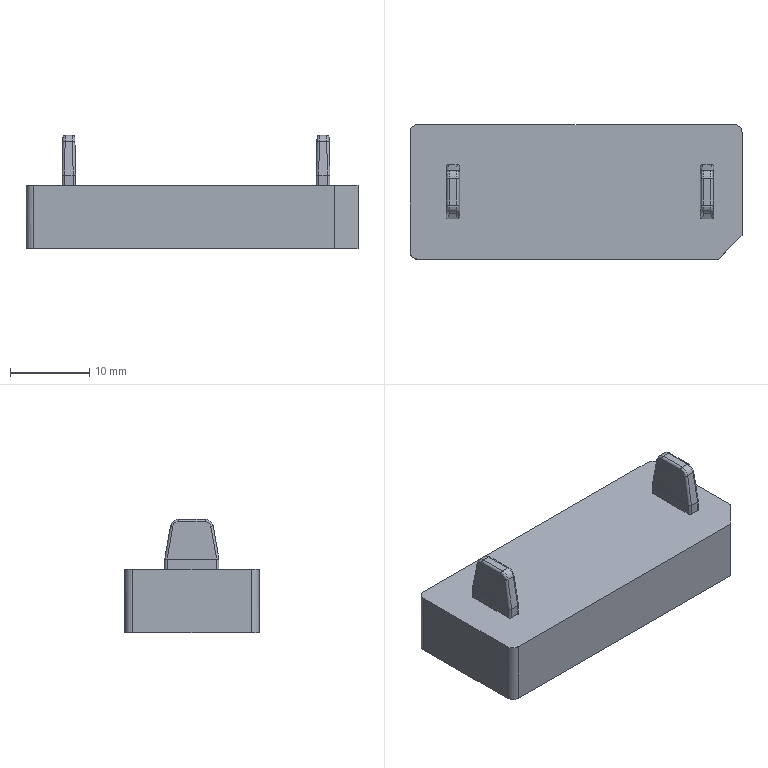NC program | PowerMill | posted by the shop | part box 42 x 17 x 14.346 mm
Lines 3988 to 5032 of 50900:
( TOOL ID   R1_2 )
( TOOL DIA. 2. TIP RAD 1. LENGTH 57. )
( Z = -2.15 )
T4 M6
T5
G91 G28 Z0
G0 G90 G54
M08
S18000 M3
X0 Y0 M8
G43 Z10.796 H4
X17.949 Y-3.022
Z-.902
G1 Z-2.102 F1200
X17.941 Y-3.03 Z-2.084 F2000
X17.924 Y-3.048 Z-2.051
X17.9 Y-3.071 Z-2.022
X17.871 Y-3.1 Z-1.995
X17.836 Y-3.136 Z-1.972
X17.82 Y-3.151 Z-1.974
X17.787 Y-3.185 Z-1.984
X17.755 Y-3.217 Z-2.002
X17.725 Y-3.246 Z-2.027
X17.699 Y-3.272 Z-2.059
X17.567 Y-3.353 Z-2.043
X17.603 Y-3.318 Z-1.96
X17.63 Y-3.29 Z-1.904
X17.656 Y-3.264 Z-1.861
X17.683 Y-3.238 Z-1.827
X17.71 Y-3.21 Z-1.801
X17.74 Y-3.181 Z-1.782
X17.771 Y-3.15 Z-1.77
X17.78 Y-3.14 Z-1.767
X17.869 Y-3.051 Z-1.781
X17.897 Y-3.023 Z-1.802
X17.923 Y-2.998 Z-1.83
X17.946 Y-2.974 Z-1.864
X17.968 Y-2.953 Z-1.907
X17.987 Y-2.933 Z-1.959
X18.006 Y-2.914 Z-2.024
X18.027 Y-2.894 Z-2.112
X18.029 Y-2.891 Z-2.122
X18.07 Y-2.799 Z-2.132
X18.063 Y-2.806 Z-2.079
X18.049 Y-2.821 Z-1.986
X18.033 Y-2.837 Z-1.913
X18.015 Y-2.855 Z-1.851
X17.994 Y-2.876 Z-1.797
X17.972 Y-2.897 Z-1.754
X17.947 Y-2.923 Z-1.716
X17.918 Y-2.952 Z-1.684
X17.886 Y-2.984 Z-1.659
X17.852 Y-3.018 Z-1.641
X17.817 Y-3.052 Z-1.631
X17.782 Y-3.087 Z-1.629
X17.748 Y-3.122 Z-1.635
X17.715 Y-3.155 Z-1.648
X17.678 Y-3.192 Z-1.669
X17.643 Y-3.226 Z-1.695
X17.612 Y-3.258 Z-1.727
X17.583 Y-3.287 Z-1.766
X17.556 Y-3.314 Z-1.811
X17.531 Y-3.339 Z-1.866
X17.506 Y-3.364 Z-1.933
X17.477 Y-3.393 Z-2.025
X17.396 Y-3.422 Z-2.013
X17.423 Y-3.395 Z-1.917
X17.449 Y-3.37 Z-1.839
X17.475 Y-3.344 Z-1.777
X17.501 Y-3.318 Z-1.726
X17.519 Y-3.3 Z-1.697
X17.543 Y-3.276 Z-1.663
X17.579 Y-3.24 Z-1.619
X17.608 Y-3.211 Z-1.591
X17.631 Y-3.188 Z-1.573
X17.656 Y-3.163 Z-1.558
X17.684 Y-3.135 Z-1.544
X17.715 Y-3.104 Z-1.53
X17.744 Y-3.075 Z-1.523
X17.772 Y-3.046 Z-1.521
X17.801 Y-3.017 Z-1.523
X17.827 Y-2.991 Z-1.529
X17.858 Y-2.96 Z-1.542
X17.894 Y-2.924 Z-1.56
X17.928 Y-2.89 Z-1.59
X17.959 Y-2.859 Z-1.625
X17.987 Y-2.831 Z-1.668
X18.012 Y-2.806 Z-1.716
X18.035 Y-2.784 Z-1.773
X18.054 Y-2.765 Z-1.838
X18.071 Y-2.748 Z-1.913
X18.085 Y-2.734 Z-2.001
X18.097 Y-2.722 Z-2.108
X18.099 Y-2.72 Z-2.134
X18.117 Y-2.651 Z-2.137
X18.113 Y-2.654 Z-2.082
X18.103 Y-2.664 Z-1.97
X18.091 Y-2.677 Z-1.878
X18.076 Y-2.692 Z-1.799
X18.058 Y-2.71 Z-1.732
X18.035 Y-2.733 Z-1.669
X18.009 Y-2.758 Z-1.614
X17.981 Y-2.787 Z-1.565
X17.949 Y-2.818 Z-1.524
X17.916 Y-2.852 Z-1.491
X17.881 Y-2.887 Z-1.465
X17.844 Y-2.924 Z-1.446
X17.805 Y-2.963 Z-1.434
X17.765 Y-3.003 Z-1.429
X17.723 Y-3.045 Z-1.432
X17.68 Y-3.088 Z-1.443
X17.638 Y-3.13 Z-1.461
X17.596 Y-3.172 Z-1.488
X17.554 Y-3.214 Z-1.523
X17.514 Y-3.254 Z-1.566
X17.477 Y-3.291 Z-1.615
X17.444 Y-3.324 Z-1.667
X17.414 Y-3.354 Z-1.724
X17.387 Y-3.381 Z-1.789
X17.363 Y-3.405 Z-1.862
X17.342 Y-3.426 Z-1.94
X17.324 Y-3.444 Z-2.019
X17.256 Y-3.461 Z-2.025
X17.278 Y-3.439 Z-1.925
X17.302 Y-3.415 Z-1.835
X17.329 Y-3.388 Z-1.753
X17.358 Y-3.359 Z-1.681
X17.39 Y-3.327 Z-1.616
X17.425 Y-3.292 Z-1.558
X17.463 Y-3.254 Z-1.507
X17.504 Y-3.213 Z-1.464
X17.548 Y-3.169 Z-1.426
X17.594 Y-3.123 Z-1.395
X17.638 Y-3.078 Z-1.373
X17.683 Y-3.034 Z-1.358
X17.727 Y-2.99 Z-1.35
X17.77 Y-2.947 Z-1.351
X17.812 Y-2.904 Z-1.359
X17.853 Y-2.864 Z-1.374
X17.893 Y-2.824 Z-1.397
X17.93 Y-2.787 Z-1.428
X17.964 Y-2.753 Z-1.466
X17.996 Y-2.721 Z-1.511
X18.025 Y-2.692 Z-1.562
X18.05 Y-2.667 Z-1.619
X18.071 Y-2.646 Z-1.682
X18.088 Y-2.629 Z-1.749
X18.102 Y-2.615 Z-1.825
X18.115 Y-2.602 Z-1.919
X18.125 Y-2.592 Z-2.028
X18.13 Y-2.587 Z-2.108
X18.137 Y-2.529 Z-2.075
Z-2.065
X18.13 Y-2.536 Z-1.951
X18.12 Y-2.546 Z-1.846
X18.107 Y-2.559 Z-1.755
X18.091 Y-2.575 Z-1.675
X18.071 Y-2.595 Z-1.604
X18.048 Y-2.618 Z-1.541
X18.022 Y-2.644 Z-1.486
X17.993 Y-2.673 Z-1.437
X17.961 Y-2.705 Z-1.395
X17.926 Y-2.74 Z-1.36
X17.888 Y-2.778 Z-1.33
X17.847 Y-2.819 Z-1.306
X17.805 Y-2.861 Z-1.289
X17.761 Y-2.905 Z-1.28
X17.716 Y-2.95 Z-1.279
X17.669 Y-2.997 Z-1.285
X17.621 Y-3.045 Z-1.3
X17.574 Y-3.093 Z-1.322
X17.526 Y-3.14 Z-1.353
X17.48 Y-3.186 Z-1.392
X17.436 Y-3.23 Z-1.437
X17.395 Y-3.272 Z-1.488
X17.357 Y-3.309 Z-1.543
X17.322 Y-3.344 Z-1.604
X17.291 Y-3.375 Z-1.671
X17.264 Y-3.403 Z-1.746
X17.238 Y-3.428 Z-1.829
X17.215 Y-3.451 Z-1.924
X17.194 Y-3.472 Z-2.03
X17.139 Y-3.476 Z-2.024
X17.151 Y-3.465 Z-1.964
X17.162 Y-3.453 Z-1.903
X17.175 Y-3.44 Z-1.843
X17.19 Y-3.425 Z-1.784
X17.209 Y-3.406 Z-1.727
X17.23 Y-3.386 Z-1.672
X17.251 Y-3.364 Z-1.617
X17.285 Y-3.33 Z-1.546
X17.323 Y-3.293 Z-1.481
X17.363 Y-3.252 Z-1.422
X17.407 Y-3.208 Z-1.37
X17.453 Y-3.162 Z-1.325
X17.501 Y-3.114 Z-1.288
X17.551 Y-3.064 Z-1.258
X17.602 Y-3.013 Z-1.236
X17.651 Y-2.964 Z-1.222
X17.7 Y-2.915 Z-1.216
X17.748 Y-2.867 Z-1.217
X17.795 Y-2.82 Z-1.226
X17.84 Y-2.776 Z-1.243
X17.882 Y-2.733 Z-1.267
X17.923 Y-2.692 Z-1.298
X17.96 Y-2.655 Z-1.335
X17.994 Y-2.621 Z-1.38
X18.024 Y-2.591 Z-1.43
X18.051 Y-2.564 Z-1.486
X18.075 Y-2.54 Z-1.55
X18.095 Y-2.52 Z-1.621
X18.112 Y-2.504 Z-1.7
X18.124 Y-2.491 Z-1.787
X18.134 Y-2.481 Z-1.885
X18.14 Y-2.475 Z-1.994
X18.142 Y-2.473 Z-2.044
X18.145 Y-2.42 Z-2.007
X18.141 Y-2.423 Z-1.915
X18.134 Y-2.43 Z-1.801
X18.123 Y-2.441 Z-1.704
X18.109 Y-2.455 Z-1.619
X18.091 Y-2.473 Z-1.544
X18.07 Y-2.494 Z-1.477
X18.046 Y-2.519 Z-1.417
X18.018 Y-2.546 Z-1.364
X17.987 Y-2.578 Z-1.317
X17.952 Y-2.612 Z-1.275
X17.914 Y-2.65 Z-1.24
X17.873 Y-2.691 Z-1.209
X17.828 Y-2.736 Z-1.185
X17.782 Y-2.783 Z-1.168
X17.733 Y-2.831 Z-1.158
X17.684 Y-2.881 Z-1.156
X17.633 Y-2.931 Z-1.162
X17.582 Y-2.983 Z-1.176
X17.53 Y-3.034 Z-1.198
X17.479 Y-3.085 Z-1.228
X17.429 Y-3.135 Z-1.266
X17.38 Y-3.184 Z-1.312
X17.334 Y-3.231 Z-1.365
X17.29 Y-3.274 Z-1.425
X17.254 Y-3.31 Z-1.484
X17.222 Y-3.342 Z-1.544
X17.193 Y-3.371 Z-1.607
X17.166 Y-3.398 Z-1.676
X17.142 Y-3.422 Z-1.754
X17.119 Y-3.445 Z-1.844
X17.101 Y-3.463 Z-1.933
X17.085 Y-3.479 Z-2.02
X17.035 Z-2.016
X17.052 Y-3.461 Z-1.913
X17.073 Y-3.44 Z-1.813
X17.097 Y-3.416 Z-1.721
X17.124 Y-3.389 Z-1.637
X17.154 Y-3.359 Z-1.561
X17.188 Y-3.326 Z-1.492
X17.225 Y-3.289 Z-1.427
X17.265 Y-3.248 Z-1.365
X17.31 Y-3.204 Z-1.306
X17.357 Y-3.156 Z-1.254
X17.407 Y-3.106 Z-1.209
X17.459 Y-3.054 Z-1.172
X17.513 Y-3. Z-1.142
X17.569 Y-2.945 Z-1.12
X17.621 Y-2.893 Z-1.107
X17.673 Y-2.84 Z-1.101
X17.725 Y-2.788 Z-1.104
X17.776 Y-2.738 Z-1.115
X17.824 Y-2.689 Z-1.133
X17.87 Y-2.643 Z-1.158
X17.913 Y-2.601 Z-1.189
X17.952 Y-2.561 Z-1.227
X17.988 Y-2.526 Z-1.27
X18.02 Y-2.494 Z-1.32
X18.048 Y-2.465 Z-1.374
X18.073 Y-2.44 Z-1.435
X18.094 Y-2.419 Z-1.501
X18.111 Y-2.402 Z-1.575
X18.125 Y-2.388 Z-1.657
X18.135 Y-2.378 Z-1.751
X18.142 Y-2.371 Z-1.862
X18.146 Y-2.368 Z-1.965
X18.145 Y-2.317 Z-1.925
Y-2.318 Z-1.915
X18.142 Y-2.321 Z-1.792
X18.135 Y-2.327 Z-1.69
X18.125 Y-2.338 Z-1.6
X18.111 Y-2.352 Z-1.521
X18.093 Y-2.37 Z-1.449
X18.071 Y-2.391 Z-1.385
X18.046 Y-2.417 Z-1.326
X18.017 Y-2.446 Z-1.273
X17.984 Y-2.478 Z-1.225
X17.948 Y-2.515 Z-1.182
X17.907 Y-2.555 Z-1.143
X17.863 Y-2.599 Z-1.11
X17.817 Y-2.646 Z-1.084
X17.768 Y-2.695 Z-1.065
X17.717 Y-2.745 Z-1.054
X17.664 Y-2.798 Z-1.05
X17.611 Y-2.852 Z-1.054
X17.556 Y-2.906 Z-1.067
X17.502 Y-2.961 Z-1.087
X17.447 Y-3.015 Z-1.115
X17.394 Y-3.069 Z-1.151
X17.342 Y-3.121 Z-1.195
X17.292 Y-3.171 Z-1.246
X17.251 Y-3.212 Z-1.296
X17.21 Y-3.252 Z-1.35
X17.173 Y-3.289 Z-1.41
X17.137 Y-3.326 Z-1.478
X17.105 Y-3.357 Z-1.548
X17.078 Y-3.384 Z-1.617
X17.053 Y-3.409 Z-1.691
X17.031 Y-3.432 Z-1.774
X17.009 Y-3.453 Z-1.875
X16.984 Y-3.478 Z-2.011
X16.934 Y-3.477 Z-2.006
X16.96 Y-3.452 Z-1.869
X16.984 Y-3.428 Z-1.761
X17.009 Y-3.403 Z-1.669
X17.037 Y-3.375 Z-1.586
X17.072 Y-3.34 Z-1.5
X17.111 Y-3.3 Z-1.42
X17.155 Y-3.257 Z-1.345
X17.201 Y-3.21 Z-1.276
X17.251 Y-3.161 Z-1.215
X17.303 Y-3.109 Z-1.161
X17.356 Y-3.055 Z-1.115
X17.411 Y-3.001 Z-1.077
X17.466 Y-2.945 Z-1.048
X17.522 Y-2.889 Z-1.026
X17.579 Y-2.833 Z-1.012
X17.635 Y-2.776 Z-1.005
X17.691 Y-2.72 Z-1.007
X17.742 Y-2.669 Z-1.016
X17.793 Y-2.619 Z-1.032
X17.842 Y-2.57 Z-1.056
X17.888 Y-2.523 Z-1.087
X17.932 Y-2.48 Z-1.125
X17.971 Y-2.44 Z-1.17
X18.007 Y-2.404 Z-1.219
X18.039 Y-2.372 Z-1.274
X18.066 Y-2.345 Z-1.334
X18.09 Y-2.322 Z-1.399
X18.108 Y-2.303 Z-1.468
X18.123 Y-2.289 Z-1.544
X18.133 Y-2.278 Z-1.628
X18.14 Y-2.271 Z-1.724
X18.144 Y-2.268 Z-1.84
Y-2.267 Z-1.884
X18.143 Y-2.217 Z-1.832
Z-1.822
X18.141 Y-2.219 Z-1.708
X18.136 Y-2.225 Z-1.612
X18.126 Y-2.235 Z-1.527
X18.112 Y-2.248 Z-1.45
X18.095 Y-2.266 Z-1.38
X18.072 Y-2.288 Z-1.313
X18.046 Y-2.314 Z-1.254
X18.016 Y-2.345 Z-1.198
X17.98 Y-2.38 Z-1.146
X17.941 Y-2.42 Z-1.1
X17.897 Y-2.464 Z-1.059
X17.85 Y-2.511 Z-1.025
X17.8 Y-2.56 Z-.997
X17.749 Y-2.611 Z-.978
X17.697 Y-2.664 Z-.966
X17.641 Y-2.72 Z-.961
X17.584 Y-2.777 Z-.964
X17.526 Y-2.835 Z-.975
X17.468 Y-2.892 Z-.994
X17.411 Y-2.95 Z-1.021
X17.355 Y-3.006 Z-1.056
X17.3 Y-3.061 Z-1.098
X17.247 Y-3.113 Z-1.147
X17.197 Y-3.164 Z-1.204
X17.149 Y-3.212 Z-1.267
X17.104 Y-3.257 Z-1.336
X17.062 Y-3.299 Z-1.412
X17.024 Y-3.337 Z-1.493
X16.989 Y-3.372 Z-1.579
X16.958 Y-3.402 Z-1.67
X16.931 Y-3.429 Z-1.767
X16.907 Y-3.454 Z-1.875
X16.884 Y-3.476 Z-2.001
X16.834 Y-3.475 Z-1.996
X16.859 Y-3.451 Z-1.864
X16.881 Y-3.428 Z-1.761
X16.905 Y-3.404 Z-1.675
X16.932 Y-3.378 Z-1.597
X16.97 Y-3.339 Z-1.5
X17.01 Y-3.299 Z-1.411
X17.052 Y-3.258 Z-1.332
X17.096 Y-3.214 Z-1.261
X17.142 Y-3.168 Z-1.197
X17.191 Y-3.119 Z-1.14
X17.242 Y-3.067 Z-1.088
X17.298 Y-3.012 Z-1.04
X17.355 Y-2.955 Z-1.
X17.413 Y-2.897 Z-.968
X17.471 Y-2.838 Z-.944
X17.53 Y-2.78 Z-.928
X17.588 Y-2.721 Z-.92
X17.646 Y-2.664
X17.702 Y-2.608 Z-.928
X17.756 Y-2.553 Z-.944
X17.809 Y-2.501 Z-.966
X17.858 Y-2.452 Z-.995
X17.904 Y-2.406 Z-1.031
X17.947 Y-2.363 Z-1.074
X17.986 Y-2.323 Z-1.122
X18.021 Y-2.289 Z-1.175
X18.051 Y-2.258 Z-1.233
X18.077 Y-2.233 Z-1.295
X18.098 Y-2.212 Z-1.359
X18.115 Y-2.195 Z-1.427
X18.127 Y-2.182 Z-1.502
X18.136 Y-2.173 Z-1.586
X18.141 Y-2.169 Z-1.683
X18.142 Y-2.167 Z-1.777
X18.141 Y-2.117 Z-1.723
Z-1.705
X18.139 Y-2.119 Z-1.616
X18.134 Y-2.125 Z-1.532
X18.125 Y-2.134 Z-1.454
X18.111 Y-2.148 Z-1.382
X18.093 Y-2.165 Z-1.314
X18.07 Y-2.188 Z-1.249
X18.043 Y-2.216 Z-1.187
X18.01 Y-2.249 Z-1.129
X17.973 Y-2.286 Z-1.076
X17.932 Y-2.327 Z-1.028
X17.887 Y-2.372 Z-.987
X17.839 Y-2.42 Z-.952
X17.787 Y-2.471 Z-.923
X17.734 Y-2.525 Z-.902
X17.678 Y-2.581 Z-.888
X17.621 Y-2.638 Z-.882
X17.563 Y-2.696 Z-.883
X17.505 Y-2.754 Z-.892
X17.453 Y-2.806 Z-.907
X17.392 Y-2.866 Z-.93
X17.333 Y-2.925 Z-.961
X17.276 Y-2.983 Z-1.
X17.22 Y-3.039 Z-1.047
X17.165 Y-3.094 Z-1.101
X17.112 Y-3.147 Z-1.163
X17.061 Y-3.197 Z-1.233
X17.013 Y-3.246 Z-1.311
X16.966 Y-3.292 Z-1.397
X16.923 Y-3.336 Z-1.491
X16.882 Y-3.377 Z-1.593
X16.855 Y-3.404 Z-1.672
X16.831 Y-3.428 Z-1.759
X16.808 Y-3.451 Z-1.862
X16.784 Y-3.475 Z-1.994
X16.733 Z-1.993
X16.756 Y-3.452 Z-1.869
X16.78 Y-3.428 Z-1.761
X16.807 Y-3.401 Z-1.665
X16.834 Y-3.374 Z-1.586
X16.866 Y-3.341 Z-1.503
X16.907 Y-3.301 Z-1.415
X16.955 Y-3.253 Z-1.324
X17.008 Y-3.2 Z-1.237
X17.061 Y-3.147 Z-1.16
X17.113 Y-3.095 Z-1.094
X17.163 Y-3.044 Z-1.039
X17.211 Y-2.997 Z-.996
X17.27 Y-2.937 Z-.951
X17.331 Y-2.876 Z-.914
X17.393 Y-2.815 Z-.884
X17.455 Y-2.753 Z-.863
X17.516 Y-2.691 Z-.85
X17.577 Y-2.631 Z-.845
X17.636 Y-2.572 Z-.848
X17.693 Y-2.515 Z-.858
X17.749 Y-2.459 Z-.876
X17.802 Y-2.406 Z-.901
X17.853 Y-2.355 Z-.934
X17.9 Y-2.308 Z-.972
X17.944 Y-2.264 Z-1.016
X17.984 Y-2.224 Z-1.067
X18.02 Y-2.187 Z-1.122
X18.052 Y-2.156 Z-1.183
X18.078 Y-2.13 Z-1.246
X18.099 Y-2.108 Z-1.312
X18.116 Y-2.092 Z-1.383
X18.129 Y-2.079 Z-1.46
X18.137 Y-2.071 Z-1.545
X18.14 Y-2.068 Z-1.639
Y-2.067 Z-1.668
Y-2.017 Z-1.645
Z-1.635
X18.138 Y-2.019 Z-1.554
X18.133 Y-2.024 Z-1.473
X18.124 Y-2.033 Z-1.398
X18.11 Y-2.047 Z-1.33
X18.092 Y-2.065 Z-1.266
X18.071 Y-2.086 Z-1.206
X18.046 Y-2.111 Z-1.148
X18.014 Y-2.143 Z-1.089
X17.977 Y-2.18 Z-1.033
X17.936 Y-2.221 Z-.983
X17.891 Y-2.266 Z-.938
X17.842 Y-2.315 Z-.9
X17.789 Y-2.367 Z-.868
X17.735 Y-2.422 Z-.843
X17.678 Y-2.479 Z-.825
X17.619 Y-2.538 Z-.814
X17.559 Y-2.598 Z-.811
X17.498 Y-2.659 Z-.815
X17.437 Y-2.72 Z-.828
X17.376 Y-2.781 Z-.848
X17.315 Y-2.842 Z-.876
X17.255 Y-2.902 Z-.913
X17.195 Y-2.962 Z-.957
X17.137 Y-3.02 Z-1.01
X17.08 Y-3.077 Z-1.07
X17.028 Y-3.128 Z-1.134
X16.971 Y-3.186 Z-1.214
X16.917 Y-3.24 Z-1.301
X16.867 Y-3.29 Z-1.393
X16.822 Y-3.335 Z-1.49
X16.781 Y-3.376 Z-1.591
X16.754 Y-3.403 Z-1.671
X16.73 Y-3.427 Z-1.758
X16.707 Y-3.45 Z-1.861
X16.682 Y-3.475 Z-1.993
X16.631 Z-1.992
X16.656 Y-3.45 Z-1.859
X16.68 Y-3.426 Z-1.753
X16.705 Y-3.401 Z-1.662
X16.731 Y-3.375 Z-1.586
X16.763 Y-3.343 Z-1.507
X16.803 Y-3.303 Z-1.421
X16.851 Y-3.255 Z-1.329
X16.908 Y-3.198 Z-1.235
X16.966 Y-3.14 Z-1.148
X17.023 Y-3.083 Z-1.074
X17.076 Y-3.03 Z-1.013
X17.126 Y-2.98 Z-.963
X17.176 Y-2.931 Z-.92
X17.228 Y-2.878 Z-.883
X17.291 Y-2.815 Z-.846
X17.354 Y-2.752 Z-.817
X17.417 Y-2.689 Z-.797
X17.48 Y-2.626 Z-.784
X17.542 Y-2.564 Z-.779
X17.602 Y-2.504 Z-.782
X17.662 Y-2.444 Z-.792
X17.721 Y-2.385 Z-.81
X17.777 Y-2.329 Z-.836
X17.83 Y-2.276 Z-.868
X17.88 Y-2.226 Z-.907
X17.926 Y-2.18 Z-.952
X17.969 Y-2.137 Z-1.002
X18.007 Y-2.099 Z-1.058
X18.04 Y-2.066 Z-1.118
X18.068 Y-2.038 Z-1.178
X18.09 Y-2.016 Z-1.241
X18.109 Y-1.997 Z-1.307
X18.123 Y-1.983 Z-1.379
X18.133 Y-1.973 Z-1.457
X18.138 Y-1.968 Z-1.544
X18.14 Y-1.966 Z-1.622
X18.139 Y-1.916 Z-1.599
Z-1.563
X18.136 Y-1.92 Z-1.473
X18.128 Y-1.927 Z-1.395
X18.117 Y-1.938 Z-1.326
X18.099 Y-1.956 Z-1.254
X18.076 Y-1.979 Z-1.184
X18.047 Y-2.008 Z-1.117
X18.014 Y-2.041 Z-1.054
X17.976 Y-2.079 Z-.996
X17.934 Y-2.121 Z-.942
X17.888 Y-2.167 Z-.894
X17.839 Y-2.216 Z-.853
X17.787 Y-2.268 Z-.819
X17.73 Y-2.325 Z-.79
X17.672 Y-2.383 Z-.769
X17.612 Y-2.443 Z-.755
X17.551 Y-2.504 Z-.749
X17.489 Y-2.566 Z-.75
X17.426 Y-2.63 Z-.759
X17.362 Y-2.693 Z-.777
X17.298 Y-2.757 Z-.802
X17.234 Y-2.821 Z-.836
X17.172 Y-2.883 Z-.877
X17.111 Y-2.944 Z-.926
X17.053 Y-3.002 Z-.982
X16.997 Y-3.058 Z-1.044
X16.931 Y-3.124 Z-1.127
X16.87 Y-3.185 Z-1.213
X16.814 Y-3.241 Z-1.303
X16.764 Y-3.291 Z-1.396
X16.719 Y-3.336 Z-1.491
X16.68 Y-3.375 Z-1.589
X16.652 Y-3.403 Z-1.67
X16.628 Y-3.427 Z-1.757
X16.605 Y-3.45 Z-1.86
X16.581 Y-3.474 Z-1.991
X16.53 Z-1.99
X16.554 Y-3.451 Z-1.861
X16.577 Y-3.428 Z-1.759
X16.601 Y-3.403 Z-1.671
X16.628 Y-3.376 Z-1.591
X16.669 Y-3.335 Z-1.491
X16.715 Y-3.289 Z-1.393
X16.766 Y-3.238 Z-1.298
X16.822 Y-3.182 Z-1.208
X16.883 Y-3.121 Z-1.122
X16.948 Y-3.056 Z-1.041
X17.017 Y-2.987 Z-.965
X17.071 Y-2.933 Z-.913
X17.131 Y-2.873 Z-.862
X17.194 Y-2.811 Z-.818
X17.257 Y-2.747 Z-.783
X17.321 Y-2.683 Z-.755
X17.386 Y-2.619 Z-.735
X17.45 Y-2.554 Z-.724
X17.514 Y-2.49 Z-.72
X17.578 Y-2.426 Z-.724
X17.641 Y-2.363 Z-.736
X17.7 Y-2.304 Z-.755
X17.757 Y-2.247 Z-.781
X17.812 Y-2.192 Z-.815
X17.865 Y-2.14 Z-.855
X17.913 Y-2.091 Z-.901
X17.957 Y-2.047 Z-.953
X17.997 Y-2.007 Z-1.01
X18.032 Y-1.972 Z-1.071
X18.062 Y-1.942 Z-1.135
X18.085 Y-1.919 Z-1.197
X18.104 Y-1.9 Z-1.26
X18.119 Y-1.885 Z-1.327
X18.13 Y-1.874 Z-1.4
X18.136 Y-1.868 Z-1.477
X18.139 Y-1.865 Z-1.554
Z-1.579
Y-1.815 Z-1.569
X18.138 Z-1.528
X18.136 Y-1.817 Z-1.466
X18.131 Y-1.822 Z-1.4
X18.122 Y-1.831 Z-1.333
X18.11 Y-1.843 Z-1.274
X18.094 Y-1.859 Z-1.217
X18.076 Y-1.877 Z-1.162
X18.053 Y-1.9 Z-1.104
X18.022 Y-1.931 Z-1.041
X17.986 Y-1.967 Z-.981
X17.945 Y-2.008 Z-.924
X17.899 Y-2.054 Z-.872
X17.849 Y-2.104 Z-.826
X17.796 Y-2.157 Z-.786
X17.741 Y-2.212 Z-.753
X17.683 Y-2.27 Z-.727
X17.622 Y-2.331 Z-.708
X17.56 Y-2.393 Z-.697
X17.496 Y-2.458 Z-.693
X17.43 Y-2.523 Z-.697
X17.364 Y-2.589 Z-.71
X17.297 Y-2.656 Z-.73
X17.231 Y-2.722 Z-.759
X17.166 Y-2.788 Z-.795
X17.113 Y-2.84 Z-.831
X17.06 Y-2.893 Z-.874
X17.002 Y-2.951 Z-.928
X16.939 Y-3.014 Z-.994
X16.871 Y-3.083 Z-1.074
X16.804 Y-3.149 Z-1.162
X16.747 Y-3.206 Z-1.246
X16.7 Y-3.253 Z-1.323
X16.662 Y-3.292 Z-1.395
X16.628 Y-3.325 Z-1.468
X16.594 Y-3.359 Z-1.549
X16.563 Y-3.39 Z-1.633
X16.536 Y-3.417 Z-1.719
X16.514 Y-3.439 Z-1.808
X16.495 Y-3.458 Z-1.898
X16.479 Y-3.474 Z-1.99
X16.428
X16.45 Y-3.452 Z-1.868
X16.474 Y-3.428 Z-1.761
X16.501 Y-3.401 Z-1.665
X16.533 Y-3.369 Z-1.574
X16.571 Y-3.331 Z-1.48
X16.615 Y-3.287 Z-1.388
X16.666 Y-3.236 Z-1.296
X16.723 Y-3.18 Z-1.206
X16.786 Y-3.116 Z-1.117
X16.855 Y-3.047 Z-1.031
X16.924 Y-2.978 Z-.954
X16.992 Y-2.91 Z-.887
X17.06 Y-2.842 Z-.83
X17.127 Y-2.775 Z-.782
X17.194 Y-2.708 Z-.742
X17.26 Y-2.642 Z-.711
X17.326 Y-2.577 Z-.689
X17.391 Y-2.512 Z-.674
X17.455 Y-2.447 Z-.668
X17.519 Y-2.383 Z-.669
X17.582 Y-2.32 Z-.678
X17.643 Y-2.259 Z-.694
X17.703 Y-2.199 Z-.717
X17.762 Y-2.141 Z-.748
X17.817 Y-2.085 Z-.786
X17.869 Y-2.033 Z-.83
X17.918 Y-1.985 Z-.88
X17.962 Y-1.941 Z-.935
X18.001 Y-1.901 Z-.995
X18.035 Y-1.867 Z-1.058
X18.065 Y-1.838 Z-1.123
X18.089 Y-1.813 Z-1.191
X18.109 Y-1.794 Z-1.263
X18.123 Y-1.779 Z-1.338
X18.133 Y-1.77 Z-1.418
X18.138 Y-1.765 Z-1.501
X18.139 Y-1.764 Z-1.559
X18.138 Y-1.713 Z-1.549
Z-1.515
X18.135 Y-1.717 Z-1.431
X18.127 Y-1.725 Z-1.353
X18.114 Y-1.737 Z-1.282
X18.098 Y-1.754 Z-1.215
X18.077 Y-1.775 Z-1.149
X18.049 Y-1.803 Z-1.078
X18.015 Y-1.836 Z-1.011
X17.977 Y-1.874 Z-.948
X17.934 Y-1.917 Z-.889
X17.888 Y-1.964 Z-.836
X17.837 Y-2.015 Z-.788
X17.783 Y-2.069 Z-.746
X17.726 Y-2.126 Z-.711
X17.666 Y-2.185 Z-.683
X17.605 Y-2.247 Z-.663
X17.541 Y-2.311 Z-.649
X17.475 Y-2.376 Z-.644
X17.409 Y-2.443 Z-.646
X17.342 Y-2.51 Z-.656
X17.277 Y-2.575 Z-.674
X17.21 Y-2.641 Z-.7
X17.142 Y-2.709 Z-.734
X17.075 Y-2.776 Z-.777
X17.011 Y-2.84 Z-.826
X16.951 Y-2.9 Z-.879
X16.871 Y-2.981 Z-.958
X16.797 Y-3.054 Z-1.039
X16.73 Y-3.122 Z-1.124
X16.668 Y-3.183 Z-1.21
X16.613 Y-3.239 Z-1.3
X16.562 Y-3.289 Z-1.392
X16.517 Y-3.334 Z-1.488
X16.477 Y-3.374 Z-1.587
X16.449 Y-3.402 Z-1.668
X16.425 Y-3.427 Z-1.756
X16.401 Y-3.45 Z-1.86
X16.377 Y-3.474 Z-1.991
X16.326 Y-3.475 Z-1.993
X16.345 Y-3.456 Z-1.885
X16.368 Y-3.433 Z-1.781
X16.395 Y-3.405 Z-1.681
X16.428 Y-3.373 Z-1.584
X16.465 Y-3.335 Z-1.489
X16.508 Y-3.292 Z-1.397
X16.557 Y-3.244 Z-1.308
X16.611 Y-3.19 Z-1.22
X16.672 Y-3.129 Z-1.134
X16.738 Y-3.062 Z-1.049
X16.795 Y-3.006 Z-.985
X16.861 Y-2.939 Z-.916
X16.939 Y-2.861 Z-.844
X17.013 Y-2.787 Z-.784
X17.079 Y-2.721 Z-.738
X17.139 Y-2.662 Z-.702
X17.195 Y-2.605 Z-.674
X17.253 Y-2.547 Z-.652
X17.322 Y-2.479 Z-.634
X17.39 Y-2.41 Z-.624
X17.458 Y-2.342 Z-.622
X17.525 Y-2.276 Z-.628
X17.59 Y-2.211 Z-.641
X17.652 Y-2.148 Z-.662
X17.713 Y-2.088 Z-.69
X17.77 Y-2.031 Z-.725
X17.825 Y-1.976 Z-.766
X17.876 Y-1.925 Z-.814
X17.924 Y-1.876 Z-.869
X17.968 Y-1.832 Z-.929
X18.008 Y-1.793 Z-.993
X18.042 Y-1.758 Z-1.061
X18.072 Y-1.729 Z-1.132
X18.096 Y-1.705 Z-1.206
X18.112 Y-1.689 Z-1.27
X18.124 Y-1.676 Z-1.336
X18.133 Y-1.668 Z-1.409
X18.137 Y-1.663 Z-1.484
X18.138 Y-1.662 Z-1.541
Y-1.612 Z-1.537
X18.136 Y-1.614 Z-1.461
X18.129 Y-1.621 Z-1.378
X18.117 Y-1.633 Z-1.298
X18.1 Y-1.65 Z-1.221
X18.077 Y-1.673 Z-1.146
X18.049 Y-1.701 Z-1.073
X18.017 Y-1.733 Z-1.006
X17.979 Y-1.771 Z-.939
X17.936 Y-1.813 Z-.877
X17.889 Y-1.86 Z-.82
X17.839 Y-1.911 Z-.769
X17.784 Y-1.965 Z-.724
X17.726 Y-2.023 Z-.685
X17.666 Y-2.084 Z-.653
X17.602 Y-2.147 Z-.629
X17.537 Y-2.213 Z-.611
X17.471 Y-2.279 Z-.602
X17.403 Y-2.346 Z-.6
X17.335 Y-2.414 Z-.607
X17.273 Y-2.476 Z-.619
X17.207 Y-2.543 Z-.641
X17.138 Y-2.611 Z-.67
X17.068 Y-2.681 Z-.709
X16.996 Y-2.753 Z-.757
X16.922 Y-2.828 Z-.816
X16.836 Y-2.913 Z-.892
X16.758 Y-2.992 Z-.97
X16.686 Y-3.063 Z-1.05
X16.621 Y-3.129 Z-1.134
X16.56 Y-3.189 Z-1.22
X16.506 Y-3.244 Z-1.308
X16.457 Y-3.292 Z-1.398
X16.414 Y-3.335 Z-1.49
X16.377 Y-3.373 Z-1.584
X16.344 Y-3.405 Z-1.682
X16.316 Y-3.433 Z-1.782
X16.293 Y-3.456 Z-1.886
X16.275 Y-3.475 Z-1.994
X16.223 Y-3.476 Z-1.999
X16.241 Y-3.457 Z-1.891
X16.264 Y-3.435 Z-1.788
X16.291 Y-3.408 Z-1.688
X16.323 Y-3.376 Z-1.591
X16.36 Y-3.339 Z-1.497
X16.403 Y-3.296 Z-1.405
X16.451 Y-3.248 Z-1.316
X16.504 Y-3.195 Z-1.23
X16.554 Y-3.144 Z-1.156
X16.611 Y-3.088 Z-1.08
X16.67 Y-3.029 Z-1.009
X16.735 Y-2.964 Z-.94
X16.799 Y-2.9 Z-.879
X16.866 Y-2.833 Z-.822
X16.923 Y-2.776 Z-.776
X16.991 Y-2.708 Z-.725
X17.06 Y-2.639 Z-.68
X17.127 Y-2.572 Z-.645
X17.191 Y-2.507 Z-.618
X17.255 Y-2.444 Z-.6
X17.317 Y-2.381 Z-.588
X17.38 Y-2.318 Z-.582
X17.445 Y-2.253
X17.512 Y-2.187 Z-.59
X17.577 Y-2.121 Z-.606
X17.641 Y-2.058 Z-.629
X17.702 Y-1.996 Z-.66
X17.761 Y-1.938 Z-.698
X17.817 Y-1.882 Z-.742
X17.869 Y-1.83 Z-.793
X17.917 Y-1.781 Z-.849
X17.962 Y-1.736 Z-.912
X18.003 Y-1.696 Z-.979
X18.038 Y-1.66 Z-1.049
X18.068 Y-1.63 Z-1.122
X18.093 Y-1.606 Z-1.198
X18.112 Y-1.587 Z-1.275
X18.126 Y-1.573 Z-1.355
X18.135 Y-1.564 Z-1.437
X18.138 Y-1.561 Z-1.52
Z-1.532
Y-1.51 Z-1.527
X18.137 Y-1.511 Z-1.488
X18.134 Y-1.514 Z-1.427
X18.129 Y-1.519 Z-1.367
X18.119 Y-1.528 Z-1.307
X18.106 Y-1.542 Z-1.25
X18.091 Y-1.557 Z-1.193
X18.073 Y-1.575 Z-1.138
X18.042 Y-1.605 Z-1.061
X18.007 Y-1.64 Z-.987
X17.967 Y-1.68 Z-.918
X17.923 Y-1.725 Z-.853
X17.875 Y-1.773 Z-.794
X17.823 Y-1.825 Z-.741
X17.768 Y-1.88 Z-.695
X17.708 Y-1.94 Z-.654
X17.646 Y-2.002 Z-.621
X17.581 Y-2.066 Z-.594
X17.516 Y-2.132 Z-.576
X17.448 Y-2.2 Z-.565
X17.38 Y-2.268 Z-.561
X17.31 Y-2.337 Z-.566
X17.241 Y-2.407 Z-.579
X17.171 Y-2.477 Z-.6
X17.109 Y-2.539 Z-.625
X17.048 Y-2.6 Z-.657
X16.983 Y-2.665 Z-.696
X16.909 Y-2.739 Z-.747
X16.828 Y-2.82 Z-.811
X16.74 Y-2.908 Z-.888
X16.662 Y-2.986 Z-.964
X16.596 Y-3.051 Z-1.036
X16.541 Y-3.106 Z-1.102
X16.495 Y-3.153 Z-1.165
X16.45 Y-3.197 Z-1.232
X16.397 Y-3.251 Z-1.32
X16.349 Y-3.299 Z-1.411
X16.307 Y-3.341 Z-1.504
X16.27 Y-3.378 Z-1.599
X16.238 Y-3.41 Z-1.696
X16.211 Y-3.437 Z-1.796
X16.189 Y-3.459 Z-1.899
X16.171 Y-3.477 Z-2.005
X16.119 Y-3.478 Z-2.011
X16.138 Y-3.459 Z-1.906
X16.16 Y-3.437 Z-1.799
X16.181 Y-3.415 Z-1.712
X16.208 Y-3.389 Z-1.628
X16.238 Y-3.359 Z-1.547
X16.28 Y-3.317 Z-1.451
X16.327 Y-3.27 Z-1.356
X16.38 Y-3.217 Z-1.264
X16.438 Y-3.159 Z-1.175
X16.503 Y-3.094 Z-1.087
X16.574 Y-3.023 Z-1.003
X16.624 Y-2.973 Z-.949
X16.675 Y-2.922 Z-.899
X16.736 Y-2.861 Z-.845
X16.812 Y-2.785 Z-.783
X16.902 Y-2.694 Z-.717
X16.977 Y-2.62 Z-.668
X17.039 Y-2.558 Z-.632
X17.098 Y-2.499 Z-.603
X17.159 Y-2.438 Z-.579
X17.228 Y-2.369 Z-.56
X17.298 Y-2.298 Z-.548
X17.368 Y-2.229 Z-.544
X17.438 Y-2.159 Z-.548
X17.506 Y-2.091 Z-.56
X17.572 Y-2.024 Z-.58
X17.637 Y-1.96 Z-.607
X17.699 Y-1.898 Z-.641
X17.759 Y-1.838 Z-.683
X17.815 Y-1.781 Z-.731
X17.869 Y-1.728 Z-.785
X17.918 Y-1.679 Z-.845
X17.964 Y-1.633 Z-.912
X18.005 Y-1.592 Z-.982
X18.041 Y-1.556 Z-1.055
X18.071 Y-1.526 Z-1.13
X18.095 Y-1.502 Z-1.206
X18.114 Y-1.483 Z-1.284
X18.127 Y-1.47 Z-1.364
X18.135 Y-1.462 Z-1.445
X18.138 Y-1.459 Z-1.526
Y-1.408
X18.136 Y-1.41 Z-1.458
X18.129 Y-1.417 Z-1.378
X18.117 Y-1.429 Z-1.3
X18.1 Y-1.446 Z-1.223
X18.077 Y-1.469 Z-1.148
X18.049 Y-1.497 Z-1.074
X18.014 Y-1.532 Z-1.002
X17.974 Y-1.572 Z-.93
X17.928 Y-1.618 Z-.859
X17.878 Y-1.668 Z-.795
X17.825 Y-1.721 Z-.737
X17.769 Y-1.777 Z-.686
X17.711 Y-1.835 Z-.643
X17.65 Y-1.896 Z-.606
X17.588 Y-1.958 Z-.577
X17.523 Y-2.023 Z-.554
X17.459 Y-2.087 Z-.538
X17.393 Y-2.153 Z-.529
X17.327 Y-2.219 Z-.527
X17.26 Y-2.286 Z-.534
X17.191 Y-2.355 Z-.548
X17.12 Y-2.426 Z-.57
X17.046 Y-2.5 Z-.602
X16.969 Y-2.577 Z-.642
X16.885 Y-2.661 Z-.694
X16.795 Y-2.751 Z-.757
X16.722 Y-2.824 Z-.813
X16.646 Y-2.9 Z-.879
X16.568 Y-2.978 Z-.956
X16.494 Y-3.052 Z-1.037
X16.428 Y-3.117 Z-1.118
X16.372 Y-3.174 Z-1.197
X16.322 Y-3.224 Z-1.276
X16.275 Y-3.271 Z-1.358
X16.231 Y-3.315 Z-1.444
X16.192 Y-3.354 Z-1.534
X16.157 Y-3.389 Z-1.627
X16.129 Y-3.417 Z-1.722
X16.104 Y-3.442 Z-1.819
X16.084 Y-3.462 Z-1.917
X16.068 Y-3.478 Z-2.018
X16.02 Y-3.475 Z-2.019
X16.034 Y-3.461 Z-1.927
X16.051 Y-3.444 Z-1.837
X16.071 Y-3.424 Z-1.748
X16.095 Y-3.4 Z-1.661
X16.125 Y-3.37 Z-1.573
X16.159 Y-3.337 Z-1.492
X16.195 Y-3.3 Z-1.414
X16.235 Y-3.261 Z-1.339
X16.276 Y-3.219 Z-1.267
X16.328 Y-3.167 Z-1.186
X16.389 Y-3.106 Z-1.104
X16.457 Y-3.038 Z-1.02
X16.53 Y-2.965 Z-.941
X16.608 Y-2.887 Z-.867
X16.692 Y-2.803 Z-.797
X16.783 Y-2.713 Z-.73
X16.882 Y-2.614 Z-.665
X16.977 Y-2.518 Z-.61
X17.049 Y-2.446 Z-.574
X17.121 Y-2.374 Z-.547
X17.194 Y-2.301 Z-.528
X17.266 Y-2.229 Z-.516
X17.337 Y-2.158 Z-.513
X17.407 Y-2.088 Z-.518
X17.476 Y-2.019 Z-.53
X17.543 Y-1.952 Z-.55
X17.609 Y-1.887 Z-.577
X17.672 Y-1.823 Z-.612
X17.732 Y-1.763 Z-.654
X17.79 Y-1.705 Z-.703
X17.831 Y-1.664 Z-.743
X17.875 Y-1.62 Z-.792
X17.923 Y-1.572 Z-.854
X17.971 Y-1.524 Z-.926
X18.013 Y-1.482 Z-.999
X18.048 Y-1.447 Z-1.071